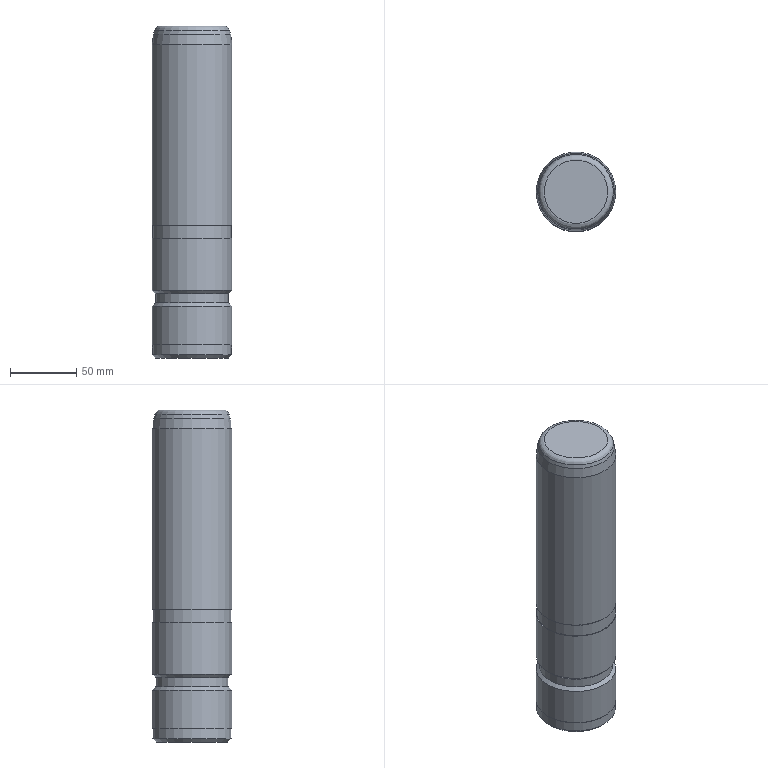Part | NX | features SGP 60-250 2 | 1 solid | 17 faces | box 60 x 60 x 250 mm | volume 697619 mm3 | cylinder 6 | plane 5 | cone 4 | sphere 1 | torus 1 | commonest cylinder face diameters 60 x3 55 x1 59 x1 59.5 x1
STEP:
#1=CARTESIAN_POINT('',(-1465.,-395.,-24.));
#2=VERTEX_POINT('',#1);
#3=CARTESIAN_POINT('',(-1495.,-395.,-24.));
#4=DIRECTION('',(0.,0.,1.));
#5=DIRECTION('',(1.,0.,0.));
#6=AXIS2_PLACEMENT_3D('',#3,#4,#5);
#7=CIRCLE('',#6,30.);
#8=EDGE_CURVE('',#2,#2,#7,.F.);
#9=ORIENTED_EDGE('',*,*,#8,.F.);
#10=EDGE_LOOP('',(#9));
#11=FACE_BOUND('',#10,.T.);
#12=CARTESIAN_POINT('',(-1525.,-395.,15.));
#13=VERTEX_POINT('',#12);
#14=CARTESIAN_POINT('',(-1495.,-395.,15.));
#15=DIRECTION('',(0.,0.,-1.));
#16=DIRECTION('',(-1.,0.,0.));
#17=AXIS2_PLACEMENT_3D('',#14,#15,#16);
#18=CIRCLE('',#17,30.);
#19=EDGE_CURVE('',#13,#13,#18,.T.);
#20=ORIENTED_EDGE('',*,*,#19,.T.);
#21=EDGE_LOOP('',(#20));
#22=FACE_BOUND('',#21,.T.);
#23=CARTESIAN_POINT('',(-1495.,-395.,-65.));
#24=DIRECTION('',(0.,0.,1.));
#25=DIRECTION('',(1.,0.,0.));
#26=AXIS2_PLACEMENT_3D('',#23,#24,#25);
#27=CYLINDRICAL_SURFACE('',#26,30.);
#28=ADVANCED_FACE('',(#11,#22),#27,.T.);
#29=CARTESIAN_POINT('',(-1465.5,-395.,15.));
#30=VERTEX_POINT('',#29);
#31=CARTESIAN_POINT('',(-1495.,-395.,15.));
#32=DIRECTION('',(0.,0.,1.));
#33=DIRECTION('',(1.,0.,0.));
#34=AXIS2_PLACEMENT_3D('',#31,#32,#33);
#35=CIRCLE('',#34,29.5);
#36=EDGE_CURVE('',#30,#30,#35,.T.);
#37=ORIENTED_EDGE('',*,*,#36,.F.);
#38=EDGE_LOOP('',(#37));
#39=FACE_BOUND('',#38,.T.);
#40=ORIENTED_EDGE('',*,*,#19,.F.);
#41=EDGE_LOOP('',(#40));
#42=FACE_BOUND('',#41,.T.);
#43=CARTESIAN_POINT('',(-1495.,-395.,15.));
#44=DIRECTION('',(0.,0.,1.));
#45=DIRECTION('',(1.,0.,0.));
#46=AXIS2_PLACEMENT_3D('',#43,#44,#45);
#47=PLANE('',#46);
#48=ADVANCED_FACE('',(#39,#42),#47,.T.);
#49=CARTESIAN_POINT('',(-1524.5,-395.,25.));
#50=VERTEX_POINT('',#49);
#51=CARTESIAN_POINT('',(-1495.,-395.,25.));
#52=DIRECTION('',(0.,0.,-1.));
#53=DIRECTION('',(-1.,0.,0.));
#54=AXIS2_PLACEMENT_3D('',#51,#52,#53);
#55=CIRCLE('',#54,29.5);
#56=EDGE_CURVE('',#50,#50,#55,.F.);
#57=ORIENTED_EDGE('',*,*,#56,.F.);
#58=EDGE_LOOP('',(#57));
#59=FACE_BOUND('',#58,.T.);
#60=ORIENTED_EDGE('',*,*,#36,.T.);
#61=EDGE_LOOP('',(#60));
#62=FACE_BOUND('',#61,.T.);
#63=CARTESIAN_POINT('',(-1495.,-395.,15.));
#64=DIRECTION('',(0.,0.,1.));
#65=DIRECTION('',(1.,0.,0.));
#66=AXIS2_PLACEMENT_3D('',#63,#64,#65);
#67=CYLINDRICAL_SURFACE('',#66,29.5);
#68=ADVANCED_FACE('',(#59,#62),#67,.T.);
#69=ORIENTED_EDGE('',*,*,#56,.T.);
#70=EDGE_LOOP('',(#69));
#71=FACE_BOUND('',#70,.T.);
#72=CARTESIAN_POINT('',(-1525.,-395.,25.));
#73=VERTEX_POINT('',#72);
#74=CARTESIAN_POINT('',(-1495.,-395.,25.));
#75=DIRECTION('',(0.,0.,-1.));
#76=DIRECTION('',(-1.,0.,0.));
#77=AXIS2_PLACEMENT_3D('',#74,#75,#76);
#78=CIRCLE('',#77,30.);
#79=EDGE_CURVE('',#73,#73,#78,.F.);
#80=ORIENTED_EDGE('',*,*,#79,.F.);
#81=EDGE_LOOP('',(#80));
#82=FACE_BOUND('',#81,.T.);
#83=CARTESIAN_POINT('',(-1495.,-395.,25.));
#84=DIRECTION('',(0.,0.,-1.));
#85=DIRECTION('',(-1.,0.,0.));
#86=AXIS2_PLACEMENT_3D('',#83,#84,#85);
#87=PLANE('',#86);
#88=ADVANCED_FACE('',(#71,#82),#87,.T.);
#89=CARTESIAN_POINT('',(-1465.,-395.,161.05));
#90=VERTEX_POINT('',#89);
#91=CARTESIAN_POINT('',(-1495.,-395.,161.05));
#92=DIRECTION('',(0.,0.,1.));
#93=DIRECTION('',(1.,0.,0.));
#94=AXIS2_PLACEMENT_3D('',#91,#92,#93);
#95=CIRCLE('',#94,30.);
#96=EDGE_CURVE('',#90,#90,#95,.F.);
#97=ORIENTED_EDGE('',*,*,#96,.T.);
#98=EDGE_LOOP('',(#97));
#99=FACE_BOUND('',#98,.T.);
#100=ORIENTED_EDGE('',*,*,#79,.T.);
#101=EDGE_LOOP('',(#100));
#102=FACE_BOUND('',#101,.T.);
#103=CARTESIAN_POINT('',(-1495.,-395.,25.));
#104=DIRECTION('',(0.,0.,1.));
#105=DIRECTION('',(1.,0.,0.));
#106=AXIS2_PLACEMENT_3D('',#103,#104,#105);
#107=CYLINDRICAL_SURFACE('',#106,30.);
#108=ADVANCED_FACE('',(#99,#102),#107,.T.);
#109=CARTESIAN_POINT('',(-1471.132,-395.,175.));
#110=VERTEX_POINT('',#109);
#111=CARTESIAN_POINT('',(-1495.,-395.,175.));
#112=DIRECTION('',(0.,0.,1.));
#113=DIRECTION('',(1.,0.,0.));
#114=AXIS2_PLACEMENT_3D('',#111,#112,#113);
#115=CIRCLE('',#114,23.868);
#116=EDGE_CURVE('',#110,#110,#115,.T.);
#117=ORIENTED_EDGE('',*,*,#116,.T.);
#118=EDGE_LOOP('',(#117));
#119=FACE_BOUND('',#118,.T.);
#120=CARTESIAN_POINT('',(-1495.,-395.,175.));
#121=DIRECTION('',(0.,0.,1.));
#122=DIRECTION('',(1.,0.,0.));
#123=AXIS2_PLACEMENT_3D('',#120,#121,#122);
#124=PLANE('',#123);
#125=ADVANCED_FACE('',(#119),#124,.T.);
#126=CARTESIAN_POINT('',(-1466.786,-395.,171.665));
#127=VERTEX_POINT('',#126);
#128=CARTESIAN_POINT('',(-1495.,-395.,171.665));
#129=DIRECTION('',(0.,0.,1.));
#130=DIRECTION('',(1.,0.,0.));
#131=AXIS2_PLACEMENT_3D('',#128,#129,#130);
#132=CIRCLE('',#131,28.214);
#133=EDGE_CURVE('',#127,#127,#132,.F.);
#134=ORIENTED_EDGE('',*,*,#133,.T.);
#135=EDGE_LOOP('',(#134));
#136=FACE_BOUND('',#135,.T.);
#137=CARTESIAN_POINT('',(-1523.978,-395.,168.815));
#138=VERTEX_POINT('',#137);
#139=CARTESIAN_POINT('',(-1495.,-395.,168.815));
#140=DIRECTION('',(0.,0.,-1.));
#141=DIRECTION('',(-1.,0.,0.));
#142=AXIS2_PLACEMENT_3D('',#139,#140,#141);
#143=CIRCLE('',#142,28.978);
#144=EDGE_CURVE('',#138,#138,#143,.F.);
#145=ORIENTED_EDGE('',*,*,#144,.T.);
#146=EDGE_LOOP('',(#145));
#147=FACE_BOUND('',#146,.T.);
#148=CARTESIAN_POINT('',(-1495.,-395.,175.));
#149=DIRECTION('',(0.,0.,-1.));
#150=DIRECTION('',(-1.,0.,0.));
#151=AXIS2_PLACEMENT_3D('',#148,#149,#150);
#152=CONICAL_SURFACE('',#151,27.321,0.2618);
#153=ADVANCED_FACE('',(#136,#147),#152,.T.);
#154=CARTESIAN_POINT('',(-1467.5,-395.,-26.5));
#155=VERTEX_POINT('',#154);
#156=CARTESIAN_POINT('',(-1495.,-395.,-26.5));
#157=DIRECTION('',(0.,0.,1.));
#158=DIRECTION('',(1.,0.,0.));
#159=AXIS2_PLACEMENT_3D('',#156,#157,#158);
#160=CIRCLE('',#159,27.5);
#161=EDGE_CURVE('',#155,#155,#160,.F.);
#162=ORIENTED_EDGE('',*,*,#161,.T.);
#163=EDGE_LOOP('',(#162));
#164=FACE_BOUND('',#163,.T.);
#165=CARTESIAN_POINT('',(-1522.5,-395.,-33.5));
#166=VERTEX_POINT('',#165);
#167=CARTESIAN_POINT('',(-1495.,-395.,-33.5));
#168=DIRECTION('',(0.,0.,-1.));
#169=DIRECTION('',(-1.,0.,0.));
#170=AXIS2_PLACEMENT_3D('',#167,#168,#169);
#171=CIRCLE('',#170,27.5);
#172=EDGE_CURVE('',#166,#166,#171,.F.);
#173=ORIENTED_EDGE('',*,*,#172,.T.);
#174=EDGE_LOOP('',(#173));
#175=FACE_BOUND('',#174,.T.);
#176=CARTESIAN_POINT('',(-1495.,-395.,-36.));
#177=DIRECTION('',(0.,0.,1.));
#178=DIRECTION('',(1.,0.,0.));
#179=AXIS2_PLACEMENT_3D('',#176,#177,#178);
#180=CYLINDRICAL_SURFACE('',#179,27.5);
#181=ADVANCED_FACE('',(#164,#175),#180,.T.);
#182=CARTESIAN_POINT('',(-1522.25,-395.,-75.));
#183=VERTEX_POINT('',#182);
#184=CARTESIAN_POINT('',(-1495.,-395.,-75.));
#185=DIRECTION('',(0.,0.,-1.));
#186=DIRECTION('',(-1.,0.,0.));
#187=AXIS2_PLACEMENT_3D('',#184,#185,#186);
#188=CIRCLE('',#187,27.25);
#189=EDGE_CURVE('',#183,#183,#188,.T.);
#190=ORIENTED_EDGE('',*,*,#189,.T.);
#191=EDGE_LOOP('',(#190));
#192=FACE_BOUND('',#191,.T.);
#193=CARTESIAN_POINT('',(-1495.,-395.,-75.));
#194=DIRECTION('',(0.,0.,-1.));
#195=DIRECTION('',(-1.,0.,0.));
#196=AXIS2_PLACEMENT_3D('',#193,#194,#195);
#197=PLANE('',#196);
#198=ADVANCED_FACE('',(#192),#197,.T.);
#199=CARTESIAN_POINT('',(-1524.75,-395.,-72.5));
#200=VERTEX_POINT('',#199);
#201=CARTESIAN_POINT('',(-1495.,-395.,-72.5));
#202=DIRECTION('',(0.,0.,-1.));
#203=DIRECTION('',(-1.,0.,0.));
#204=AXIS2_PLACEMENT_3D('',#201,#202,#203);
#205=CIRCLE('',#204,29.75);
#206=EDGE_CURVE('',#200,#200,#205,.F.);
#207=ORIENTED_EDGE('',*,*,#206,.T.);
#208=EDGE_LOOP('',(#207));
#209=FACE_BOUND('',#208,.T.);
#210=CARTESIAN_POINT('',(-1524.75,-395.,-65.));
#211=VERTEX_POINT('',#210);
#212=CARTESIAN_POINT('',(-1495.,-395.,-65.));
#213=DIRECTION('',(0.,0.,-1.));
#214=DIRECTION('',(-1.,0.,0.));
#215=AXIS2_PLACEMENT_3D('',#212,#213,#214);
#216=CIRCLE('',#215,29.75);
#217=EDGE_CURVE('',#211,#211,#216,.F.);
#218=ORIENTED_EDGE('',*,*,#217,.F.);
#219=EDGE_LOOP('',(#218));
#220=FACE_BOUND('',#219,.T.);
#221=CARTESIAN_POINT('',(-1495.,-395.,-75.));
#222=DIRECTION('',(0.,0.,1.));
#223=DIRECTION('',(1.,0.,0.));
#224=AXIS2_PLACEMENT_3D('',#221,#222,#223);
#225=CYLINDRICAL_SURFACE('',#224,29.75);
#226=ADVANCED_FACE('',(#209,#220),#225,.T.);
#227=ORIENTED_EDGE('',*,*,#217,.T.);
#228=EDGE_LOOP('',(#227));
#229=FACE_BOUND('',#228,.T.);
#230=CARTESIAN_POINT('',(-1465.,-395.,-65.));
#231=VERTEX_POINT('',#230);
#232=CARTESIAN_POINT('',(-1495.,-395.,-65.));
#233=DIRECTION('',(0.,0.,1.));
#234=DIRECTION('',(1.,0.,0.));
#235=AXIS2_PLACEMENT_3D('',#232,#233,#234);
#236=CIRCLE('',#235,30.);
#237=EDGE_CURVE('',#231,#231,#236,.T.);
#238=ORIENTED_EDGE('',*,*,#237,.F.);
#239=EDGE_LOOP('',(#238));
#240=FACE_BOUND('',#239,.T.);
#241=CARTESIAN_POINT('',(-1495.,-395.,-65.));
#242=DIRECTION('',(0.,0.,-1.));
#243=DIRECTION('',(-1.,0.,0.));
#244=AXIS2_PLACEMENT_3D('',#241,#242,#243);
#245=PLANE('',#244);
#246=ADVANCED_FACE('',(#229,#240),#245,.T.);
#247=CARTESIAN_POINT('',(-1525.,-395.,-36.));
#248=VERTEX_POINT('',#247);
#249=CARTESIAN_POINT('',(-1495.,-395.,-36.));
#250=DIRECTION('',(0.,0.,-1.));
#251=DIRECTION('',(-1.,0.,0.));
#252=AXIS2_PLACEMENT_3D('',#249,#250,#251);
#253=CIRCLE('',#252,30.);
#254=EDGE_CURVE('',#248,#248,#253,.F.);
#255=ORIENTED_EDGE('',*,*,#254,.F.);
#256=EDGE_LOOP('',(#255));
#257=FACE_BOUND('',#256,.T.);
#258=ORIENTED_EDGE('',*,*,#237,.T.);
#259=EDGE_LOOP('',(#258));
#260=FACE_BOUND('',#259,.T.);
#261=CARTESIAN_POINT('',(-1495.,-395.,-65.));
#262=DIRECTION('',(0.,0.,1.));
#263=DIRECTION('',(1.,0.,0.));
#264=AXIS2_PLACEMENT_3D('',#261,#262,#263);
#265=CYLINDRICAL_SURFACE('',#264,30.);
#266=ADVANCED_FACE('',(#257,#260),#265,.T.);
#267=ORIENTED_EDGE('',*,*,#189,.F.);
#268=EDGE_LOOP('',(#267));
#269=FACE_BOUND('',#268,.T.);
#270=ORIENTED_EDGE('',*,*,#206,.F.);
#271=EDGE_LOOP('',(#270));
#272=FACE_BOUND('',#271,.T.);
#273=CARTESIAN_POINT('',(-1495.,-395.,-72.5));
#274=DIRECTION('',(0.,0.,1.));
#275=DIRECTION('',(1.,0.,0.));
#276=AXIS2_PLACEMENT_3D('',#273,#274,#275);
#277=CONICAL_SURFACE('',#276,29.75,0.7854);
#278=ADVANCED_FACE('',(#269,#272),#277,.T.);
#279=ORIENTED_EDGE('',*,*,#254,.T.);
#280=EDGE_LOOP('',(#279));
#281=FACE_BOUND('',#280,.T.);
#282=ORIENTED_EDGE('',*,*,#172,.F.);
#283=EDGE_LOOP('',(#282));
#284=FACE_BOUND('',#283,.T.);
#285=CARTESIAN_POINT('',(-1495.,-395.,-33.5));
#286=DIRECTION('',(0.,0.,-1.));
#287=DIRECTION('',(-1.,0.,0.));
#288=AXIS2_PLACEMENT_3D('',#285,#286,#287);
#289=CONICAL_SURFACE('',#288,27.5,0.7854);
#290=ADVANCED_FACE('',(#281,#284),#289,.T.);
#291=ORIENTED_EDGE('',*,*,#8,.T.);
#292=EDGE_LOOP('',(#291));
#293=FACE_BOUND('',#292,.T.);
#294=ORIENTED_EDGE('',*,*,#161,.F.);
#295=EDGE_LOOP('',(#294));
#296=FACE_BOUND('',#295,.T.);
#297=CARTESIAN_POINT('',(-1495.,-395.,-26.5));
#298=DIRECTION('',(0.,0.,1.));
#299=DIRECTION('',(1.,0.,0.));
#300=AXIS2_PLACEMENT_3D('',#297,#298,#299);
#301=CONICAL_SURFACE('',#300,27.5,0.7854);
#302=ADVANCED_FACE('',(#293,#296),#301,.T.);
#303=ORIENTED_EDGE('',*,*,#96,.F.);
#304=EDGE_LOOP('',(#303));
#305=FACE_BOUND('',#304,.T.);
#306=ORIENTED_EDGE('',*,*,#144,.F.);
#307=EDGE_LOOP('',(#306));
#308=FACE_BOUND('',#307,.T.);
#309=CARTESIAN_POINT('',(-1495.,-395.,161.05));
#310=DIRECTION('',(0.,0.,1.));
#311=DIRECTION('',(1.,0.,0.));
#312=AXIS2_PLACEMENT_3D('',#309,#310,#311);
#313=SPHERICAL_SURFACE('',#312,30.);
#314=ADVANCED_FACE('',(#305,#308),#313,.T.);
#315=ORIENTED_EDGE('',*,*,#116,.F.);
#316=EDGE_LOOP('',(#315));
#317=FACE_BOUND('',#316,.T.);
#318=ORIENTED_EDGE('',*,*,#133,.F.);
#319=EDGE_LOOP('',(#318));
#320=FACE_BOUND('',#319,.T.);
#321=CARTESIAN_POINT('',(-1495.,-395.,170.5));
#322=DIRECTION('',(0.,0.,1.));
#323=DIRECTION('',(1.,0.,0.));
#324=AXIS2_PLACEMENT_3D('',#321,#322,#323);
#325=TOROIDAL_SURFACE('',#324,23.868,4.5);
#326=ADVANCED_FACE('',(#317,#320),#325,.T.);
#327=CLOSED_SHELL('',(#28,#48,#68,#88,#108,#125,#153,#181,#198,#226,#246,#266,#278,#290,#302,#314,#326));
#328=MANIFOLD_SOLID_BREP('',#327);
#329=(LENGTH_UNIT()NAMED_UNIT(*)SI_UNIT(.MILLI.,.METRE.));
#330=UNCERTAINTY_MEASURE_WITH_UNIT(LENGTH_MEASURE(0.00001),#329,'','');
#331=(NAMED_UNIT(*)PLANE_ANGLE_UNIT()SI_UNIT($,.RADIAN.));
#332=(NAMED_UNIT(*)SI_UNIT($,.STERADIAN.)SOLID_ANGLE_UNIT());
#333=(GEOMETRIC_REPRESENTATION_CONTEXT(3)GLOBAL_UNCERTAINTY_ASSIGNED_CONTEXT((#330))GLOBAL_UNIT_ASSIGNED_CONTEXT((#329,#331,#332))REPRESENTATION_CONTEXT('',''));
#334=ADVANCED_BREP_SHAPE_REPRESENTATION('',(#328),#333);